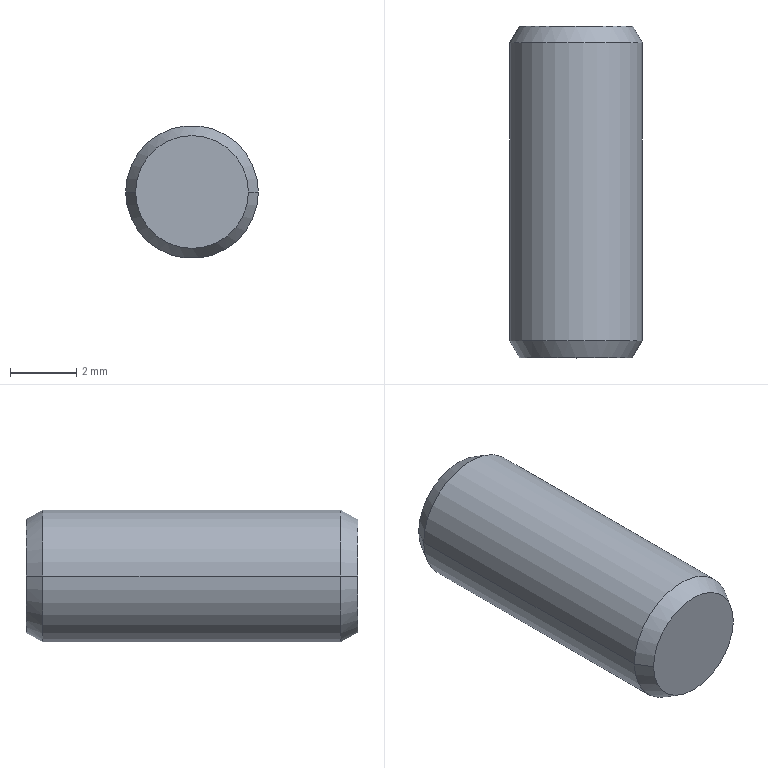Part | STEP file | 1 solid | 8 faces | box 4 x 10 x 4 mm | volume 123.869 mm3 | cone 4 | cylinder 2 | plane 2 | commonest cylinder face diameters 4 x2
STEP:
#1=CARTESIAN_POINT('',(0.,0.,0.));
#2=DIRECTION('',(0.,0.,1.));
#3=DIRECTION('',(1.,0.,0.));
#4=AXIS2_PLACEMENT_3D('',#1,#2,#3);
#5=CARTESIAN_POINT('',(-1.711,0.,0.));
#6=VERTEX_POINT('',#5);
#7=CARTESIAN_POINT('',(1.711,0.,0.));
#8=VERTEX_POINT('',#7);
#9=CARTESIAN_POINT('',(0.,0.,0.));
#10=DIRECTION('',(0.,1.,0.));
#11=DIRECTION('',(-1.,0.,0.));
#12=AXIS2_PLACEMENT_3D('',#9,#10,#11);
#13=CIRCLE('',#12,1.711);
#14=CARTESIAN_POINT('',(0.,0.,0.));
#15=DIRECTION('',(0.,-1.,0.));
#16=DIRECTION('',(1.,0.,0.));
#17=AXIS2_PLACEMENT_3D('',#14,#15,#16);
#18=CONICAL_SURFACE('',#17,1.711,0.5236);
#19=CARTESIAN_POINT('',(3.142,0.));
#20=DIRECTION('',(-1.,0.));
#21=VECTOR('',#20,1.);
#22=LINE('',#19,#21);
#23=(GEOMETRIC_REPRESENTATION_CONTEXT(2)PARAMETRIC_REPRESENTATION_CONTEXT()REPRESENTATION_CONTEXT('',''));
#24=DEFINITIONAL_REPRESENTATION('',(#22),#23);
#25=PCURVE('',#18,#24);
#26=CARTESIAN_POINT('',(0.,0.,0.));
#27=DIRECTION('',(0.,1.,0.));
#28=DIRECTION('',(-1.,0.,0.));
#29=AXIS2_PLACEMENT_3D('',#26,#27,#28);
#30=PLANE('',#29);
#31=CARTESIAN_POINT('',(0.,0.));
#32=DIRECTION('',(1.,0.));
#33=AXIS2_PLACEMENT_2D('',#31,#32);
#34=CIRCLE('',#33,1.711);
#35=(GEOMETRIC_REPRESENTATION_CONTEXT(2)PARAMETRIC_REPRESENTATION_CONTEXT()REPRESENTATION_CONTEXT('',''));
#36=DEFINITIONAL_REPRESENTATION('',(#34),#35);
#37=PCURVE('',#30,#36);
#38=SURFACE_CURVE('',#13,(#25,#37),.PCURVE_S1.);
#39=EDGE_CURVE('',#6,#8,#38,.T.);
#40=ORIENTED_EDGE('',*,*,#39,.F.);
#41=CARTESIAN_POINT('',(-2.,-0.5,0.));
#42=VERTEX_POINT('',#41);
#43=CARTESIAN_POINT('',(-1.711,0.,0.));
#44=DIRECTION('',(-0.5,-0.866,0.));
#45=VECTOR('',#44,1.);
#46=LINE('',#43,#45);
#47=CARTESIAN_POINT('',(3.142,0.));
#48=DIRECTION('',(0.,1.));
#49=VECTOR('',#48,1.);
#50=LINE('',#47,#49);
#51=(GEOMETRIC_REPRESENTATION_CONTEXT(2)PARAMETRIC_REPRESENTATION_CONTEXT()REPRESENTATION_CONTEXT('',''));
#52=DEFINITIONAL_REPRESENTATION('',(#50),#51);
#53=PCURVE('',#18,#52);
#54=CARTESIAN_POINT('',(0.,0.,0.));
#55=DIRECTION('',(0.,-1.,0.));
#56=DIRECTION('',(1.,0.,0.));
#57=AXIS2_PLACEMENT_3D('',#54,#55,#56);
#58=CONICAL_SURFACE('',#57,1.711,0.5236);
#59=CARTESIAN_POINT('',(3.142,0.));
#60=DIRECTION('',(0.,1.));
#61=VECTOR('',#60,1.);
#62=LINE('',#59,#61);
#63=(GEOMETRIC_REPRESENTATION_CONTEXT(2)PARAMETRIC_REPRESENTATION_CONTEXT()REPRESENTATION_CONTEXT('',''));
#64=DEFINITIONAL_REPRESENTATION('',(#62),#63);
#65=PCURVE('',#58,#64);
#66=SURFACE_CURVE('',#46,(#53,#65),.PCURVE_S1.);
#67=EDGE_CURVE('',#6,#42,#66,.T.);
#68=ORIENTED_EDGE('',*,*,#67,.T.);
#69=CARTESIAN_POINT('',(2.,-0.5,0.));
#70=VERTEX_POINT('',#69);
#71=CARTESIAN_POINT('',(0.,-0.5,0.));
#72=DIRECTION('',(0.,-1.,0.));
#73=DIRECTION('',(-1.,0.,0.));
#74=AXIS2_PLACEMENT_3D('',#71,#72,#73);
#75=CIRCLE('',#74,2.);
#76=CARTESIAN_POINT('',(-3.142,0.5));
#77=DIRECTION('',(1.,0.));
#78=VECTOR('',#77,1.);
#79=LINE('',#76,#78);
#80=(GEOMETRIC_REPRESENTATION_CONTEXT(2)PARAMETRIC_REPRESENTATION_CONTEXT()REPRESENTATION_CONTEXT('',''));
#81=DEFINITIONAL_REPRESENTATION('',(#79),#80);
#82=PCURVE('',#18,#81);
#83=CARTESIAN_POINT('',(0.,0.,0.));
#84=DIRECTION('',(0.,1.,0.));
#85=DIRECTION('',(-1.,0.,0.));
#86=AXIS2_PLACEMENT_3D('',#83,#84,#85);
#87=CYLINDRICAL_SURFACE('',#86,2.);
#88=CARTESIAN_POINT('',(6.283,-0.5));
#89=DIRECTION('',(-1.,0.));
#90=VECTOR('',#89,1.);
#91=LINE('',#88,#90);
#92=(GEOMETRIC_REPRESENTATION_CONTEXT(2)PARAMETRIC_REPRESENTATION_CONTEXT()REPRESENTATION_CONTEXT('',''));
#93=DEFINITIONAL_REPRESENTATION('',(#91),#92);
#94=PCURVE('',#87,#93);
#95=SURFACE_CURVE('',#75,(#82,#94),.PCURVE_S1.);
#96=EDGE_CURVE('',#70,#42,#95,.T.);
#97=ORIENTED_EDGE('',*,*,#96,.F.);
#98=CARTESIAN_POINT('',(1.711,0.,0.));
#99=DIRECTION('',(0.5,-0.866,0.));
#100=VECTOR('',#99,1.);
#101=LINE('',#98,#100);
#102=CARTESIAN_POINT('',(0.,0.));
#103=DIRECTION('',(0.,1.));
#104=VECTOR('',#103,1.);
#105=LINE('',#102,#104);
#106=(GEOMETRIC_REPRESENTATION_CONTEXT(2)PARAMETRIC_REPRESENTATION_CONTEXT()REPRESENTATION_CONTEXT('',''));
#107=DEFINITIONAL_REPRESENTATION('',(#105),#106);
#108=PCURVE('',#18,#107);
#109=CARTESIAN_POINT('',(6.283,0.));
#110=DIRECTION('',(0.,1.));
#111=VECTOR('',#110,1.);
#112=LINE('',#109,#111);
#113=(GEOMETRIC_REPRESENTATION_CONTEXT(2)PARAMETRIC_REPRESENTATION_CONTEXT()REPRESENTATION_CONTEXT('',''));
#114=DEFINITIONAL_REPRESENTATION('',(#112),#113);
#115=PCURVE('',#58,#114);
#116=SURFACE_CURVE('',#101,(#108,#115),.PCURVE_S1.);
#117=EDGE_CURVE('',#8,#70,#116,.T.);
#118=ORIENTED_EDGE('',*,*,#117,.F.);
#119=EDGE_LOOP('',(#40,#68,#97,#118));
#120=FACE_BOUND('',#119,.T.);
#121=ADVANCED_FACE('',(#120),#18,.T.);
#122=CARTESIAN_POINT('',(1.7,-10.,0.));
#123=VERTEX_POINT('',#122);
#124=CARTESIAN_POINT('',(-1.7,-10.,0.));
#125=VERTEX_POINT('',#124);
#126=CARTESIAN_POINT('',(0.,-10.,0.));
#127=DIRECTION('',(0.,-1.,0.));
#128=DIRECTION('',(1.,0.,0.));
#129=AXIS2_PLACEMENT_3D('',#126,#127,#128);
#130=CIRCLE('',#129,1.7);
#131=CARTESIAN_POINT('',(0.,-9.48,0.));
#132=DIRECTION('',(0.,1.,0.));
#133=DIRECTION('',(-1.,0.,0.));
#134=AXIS2_PLACEMENT_3D('',#131,#132,#133);
#135=CONICAL_SURFACE('',#134,2.,0.5236);
#136=CARTESIAN_POINT('',(3.142,-0.52));
#137=DIRECTION('',(-1.,0.));
#138=VECTOR('',#137,1.);
#139=LINE('',#136,#138);
#140=(GEOMETRIC_REPRESENTATION_CONTEXT(2)PARAMETRIC_REPRESENTATION_CONTEXT()REPRESENTATION_CONTEXT('',''));
#141=DEFINITIONAL_REPRESENTATION('',(#139),#140);
#142=PCURVE('',#135,#141);
#143=CARTESIAN_POINT('',(0.,-10.,0.));
#144=DIRECTION('',(0.,-1.,0.));
#145=DIRECTION('',(1.,0.,0.));
#146=AXIS2_PLACEMENT_3D('',#143,#144,#145);
#147=PLANE('',#146);
#148=CARTESIAN_POINT('',(0.,0.));
#149=DIRECTION('',(1.,0.));
#150=AXIS2_PLACEMENT_2D('',#148,#149);
#151=CIRCLE('',#150,1.7);
#152=(GEOMETRIC_REPRESENTATION_CONTEXT(2)PARAMETRIC_REPRESENTATION_CONTEXT()REPRESENTATION_CONTEXT('',''));
#153=DEFINITIONAL_REPRESENTATION('',(#151),#152);
#154=PCURVE('',#147,#153);
#155=SURFACE_CURVE('',#130,(#142,#154),.PCURVE_S1.);
#156=EDGE_CURVE('',#123,#125,#155,.T.);
#157=ORIENTED_EDGE('',*,*,#156,.F.);
#158=CARTESIAN_POINT('',(2.,-9.48,0.));
#159=VERTEX_POINT('',#158);
#160=CARTESIAN_POINT('',(2.,-9.48,0.));
#161=DIRECTION('',(0.5,0.866,0.));
#162=VECTOR('',#161,1.);
#163=LINE('',#160,#162);
#164=CARTESIAN_POINT('',(3.142,0.));
#165=DIRECTION('',(0.,1.));
#166=VECTOR('',#165,1.);
#167=LINE('',#164,#166);
#168=(GEOMETRIC_REPRESENTATION_CONTEXT(2)PARAMETRIC_REPRESENTATION_CONTEXT()REPRESENTATION_CONTEXT('',''));
#169=DEFINITIONAL_REPRESENTATION('',(#167),#168);
#170=PCURVE('',#135,#169);
#171=CARTESIAN_POINT('',(0.,-9.48,0.));
#172=DIRECTION('',(0.,1.,0.));
#173=DIRECTION('',(-1.,0.,0.));
#174=AXIS2_PLACEMENT_3D('',#171,#172,#173);
#175=CONICAL_SURFACE('',#174,2.,0.5236);
#176=CARTESIAN_POINT('',(3.142,0.));
#177=DIRECTION('',(0.,1.));
#178=VECTOR('',#177,1.);
#179=LINE('',#176,#178);
#180=(GEOMETRIC_REPRESENTATION_CONTEXT(2)PARAMETRIC_REPRESENTATION_CONTEXT()REPRESENTATION_CONTEXT('',''));
#181=DEFINITIONAL_REPRESENTATION('',(#179),#180);
#182=PCURVE('',#175,#181);
#183=SURFACE_CURVE('',#163,(#170,#182),.PCURVE_S1.);
#184=EDGE_CURVE('',#123,#159,#183,.T.);
#185=ORIENTED_EDGE('',*,*,#184,.T.);
#186=CARTESIAN_POINT('',(-2.,-9.48,0.));
#187=VERTEX_POINT('',#186);
#188=CARTESIAN_POINT('',(0.,-9.48,0.));
#189=DIRECTION('',(0.,1.,0.));
#190=DIRECTION('',(1.,0.,0.));
#191=AXIS2_PLACEMENT_3D('',#188,#189,#190);
#192=CIRCLE('',#191,2.);
#193=CARTESIAN_POINT('',(-3.142,0.));
#194=DIRECTION('',(1.,0.));
#195=VECTOR('',#194,1.);
#196=LINE('',#193,#195);
#197=(GEOMETRIC_REPRESENTATION_CONTEXT(2)PARAMETRIC_REPRESENTATION_CONTEXT()REPRESENTATION_CONTEXT('',''));
#198=DEFINITIONAL_REPRESENTATION('',(#196),#197);
#199=PCURVE('',#135,#198);
#200=CARTESIAN_POINT('',(-3.142,-9.48));
#201=DIRECTION('',(1.,0.));
#202=VECTOR('',#201,1.);
#203=LINE('',#200,#202);
#204=(GEOMETRIC_REPRESENTATION_CONTEXT(2)PARAMETRIC_REPRESENTATION_CONTEXT()REPRESENTATION_CONTEXT('',''));
#205=DEFINITIONAL_REPRESENTATION('',(#203),#204);
#206=PCURVE('',#87,#205);
#207=SURFACE_CURVE('',#192,(#199,#206),.PCURVE_S1.);
#208=EDGE_CURVE('',#187,#159,#207,.T.);
#209=ORIENTED_EDGE('',*,*,#208,.F.);
#210=CARTESIAN_POINT('',(-2.,-9.48,0.));
#211=DIRECTION('',(-0.5,0.866,0.));
#212=VECTOR('',#211,1.);
#213=LINE('',#210,#212);
#214=CARTESIAN_POINT('',(0.,0.));
#215=DIRECTION('',(0.,1.));
#216=VECTOR('',#215,1.);
#217=LINE('',#214,#216);
#218=(GEOMETRIC_REPRESENTATION_CONTEXT(2)PARAMETRIC_REPRESENTATION_CONTEXT()REPRESENTATION_CONTEXT('',''));
#219=DEFINITIONAL_REPRESENTATION('',(#217),#218);
#220=PCURVE('',#135,#219);
#221=CARTESIAN_POINT('',(6.283,0.));
#222=DIRECTION('',(0.,1.));
#223=VECTOR('',#222,1.);
#224=LINE('',#221,#223);
#225=(GEOMETRIC_REPRESENTATION_CONTEXT(2)PARAMETRIC_REPRESENTATION_CONTEXT()REPRESENTATION_CONTEXT('',''));
#226=DEFINITIONAL_REPRESENTATION('',(#224),#225);
#227=PCURVE('',#175,#226);
#228=SURFACE_CURVE('',#213,(#220,#227),.PCURVE_S1.);
#229=EDGE_CURVE('',#125,#187,#228,.T.);
#230=ORIENTED_EDGE('',*,*,#229,.F.);
#231=EDGE_LOOP('',(#157,#185,#209,#230));
#232=FACE_BOUND('',#231,.T.);
#233=ADVANCED_FACE('',(#232),#135,.T.);
#234=ORIENTED_EDGE('',*,*,#208,.T.);
#235=CARTESIAN_POINT('',(2.,0.,0.));
#236=DIRECTION('',(0.,1.,0.));
#237=VECTOR('',#236,1.);
#238=LINE('',#235,#237);
#239=CARTESIAN_POINT('',(3.142,0.));
#240=DIRECTION('',(0.,1.));
#241=VECTOR('',#240,1.);
#242=LINE('',#239,#241);
#243=(GEOMETRIC_REPRESENTATION_CONTEXT(2)PARAMETRIC_REPRESENTATION_CONTEXT()REPRESENTATION_CONTEXT('',''));
#244=DEFINITIONAL_REPRESENTATION('',(#242),#243);
#245=PCURVE('',#87,#244);
#246=CARTESIAN_POINT('',(0.,0.,0.));
#247=DIRECTION('',(0.,1.,0.));
#248=DIRECTION('',(-1.,0.,0.));
#249=AXIS2_PLACEMENT_3D('',#246,#247,#248);
#250=CYLINDRICAL_SURFACE('',#249,2.);
#251=CARTESIAN_POINT('',(3.142,0.));
#252=DIRECTION('',(0.,1.));
#253=VECTOR('',#252,1.);
#254=LINE('',#251,#253);
#255=(GEOMETRIC_REPRESENTATION_CONTEXT(2)PARAMETRIC_REPRESENTATION_CONTEXT()REPRESENTATION_CONTEXT('',''));
#256=DEFINITIONAL_REPRESENTATION('',(#254),#255);
#257=PCURVE('',#250,#256);
#258=SURFACE_CURVE('',#238,(#245,#257),.PCURVE_S1.);
#259=EDGE_CURVE('',#159,#70,#258,.T.);
#260=ORIENTED_EDGE('',*,*,#259,.T.);
#261=ORIENTED_EDGE('',*,*,#96,.T.);
#262=CARTESIAN_POINT('',(-2.,0.,0.));
#263=DIRECTION('',(0.,1.,0.));
#264=VECTOR('',#263,1.);
#265=LINE('',#262,#264);
#266=CARTESIAN_POINT('',(0.,0.));
#267=DIRECTION('',(0.,1.));
#268=VECTOR('',#267,1.);
#269=LINE('',#266,#268);
#270=(GEOMETRIC_REPRESENTATION_CONTEXT(2)PARAMETRIC_REPRESENTATION_CONTEXT()REPRESENTATION_CONTEXT('',''));
#271=DEFINITIONAL_REPRESENTATION('',(#269),#270);
#272=PCURVE('',#87,#271);
#273=CARTESIAN_POINT('',(6.283,0.));
#274=DIRECTION('',(0.,1.));
#275=VECTOR('',#274,1.);
#276=LINE('',#273,#275);
#277=(GEOMETRIC_REPRESENTATION_CONTEXT(2)PARAMETRIC_REPRESENTATION_CONTEXT()REPRESENTATION_CONTEXT('',''));
#278=DEFINITIONAL_REPRESENTATION('',(#276),#277);
#279=PCURVE('',#250,#278);
#280=SURFACE_CURVE('',#265,(#272,#279),.PCURVE_S1.);
#281=EDGE_CURVE('',#187,#42,#280,.T.);
#282=ORIENTED_EDGE('',*,*,#281,.F.);
#283=EDGE_LOOP('',(#234,#260,#261,#282));
#284=FACE_BOUND('',#283,.T.);
#285=ADVANCED_FACE('',(#284),#87,.T.);
#286=CARTESIAN_POINT('',(0.,-10.,0.));
#287=DIRECTION('',(0.,-1.,0.));
#288=DIRECTION('',(1.,0.,0.));
#289=AXIS2_PLACEMENT_3D('',#286,#287,#288);
#290=CIRCLE('',#289,1.7);
#291=CARTESIAN_POINT('',(0.,0.));
#292=DIRECTION('',(1.,0.));
#293=AXIS2_PLACEMENT_2D('',#291,#292);
#294=CIRCLE('',#293,1.7);
#295=(GEOMETRIC_REPRESENTATION_CONTEXT(2)PARAMETRIC_REPRESENTATION_CONTEXT()REPRESENTATION_CONTEXT('',''));
#296=DEFINITIONAL_REPRESENTATION('',(#294),#295);
#297=PCURVE('',#147,#296);
#298=CARTESIAN_POINT('',(9.425,-0.52));
#299=DIRECTION('',(-1.,0.));
#300=VECTOR('',#299,1.);
#301=LINE('',#298,#300);
#302=(GEOMETRIC_REPRESENTATION_CONTEXT(2)PARAMETRIC_REPRESENTATION_CONTEXT()REPRESENTATION_CONTEXT('',''));
#303=DEFINITIONAL_REPRESENTATION('',(#301),#302);
#304=PCURVE('',#175,#303);
#305=SURFACE_CURVE('',#290,(#297,#304),.PCURVE_S1.);
#306=EDGE_CURVE('',#125,#123,#305,.T.);
#307=ORIENTED_EDGE('',*,*,#306,.T.);
#308=ORIENTED_EDGE('',*,*,#156,.T.);
#309=EDGE_LOOP('',(#307,#308));
#310=FACE_BOUND('',#309,.T.);
#311=ADVANCED_FACE('',(#310),#147,.T.);
#312=ORIENTED_EDGE('',*,*,#259,.F.);
#313=CARTESIAN_POINT('',(0.,-9.48,0.));
#314=DIRECTION('',(0.,1.,0.));
#315=DIRECTION('',(1.,0.,0.));
#316=AXIS2_PLACEMENT_3D('',#313,#314,#315);
#317=CIRCLE('',#316,2.);
#318=CARTESIAN_POINT('',(3.142,-9.48));
#319=DIRECTION('',(1.,0.));
#320=VECTOR('',#319,1.);
#321=LINE('',#318,#320);
#322=(GEOMETRIC_REPRESENTATION_CONTEXT(2)PARAMETRIC_REPRESENTATION_CONTEXT()REPRESENTATION_CONTEXT('',''));
#323=DEFINITIONAL_REPRESENTATION('',(#321),#322);
#324=PCURVE('',#250,#323);
#325=CARTESIAN_POINT('',(3.142,0.));
#326=DIRECTION('',(1.,0.));
#327=VECTOR('',#326,1.);
#328=LINE('',#325,#327);
#329=(GEOMETRIC_REPRESENTATION_CONTEXT(2)PARAMETRIC_REPRESENTATION_CONTEXT()REPRESENTATION_CONTEXT('',''));
#330=DEFINITIONAL_REPRESENTATION('',(#328),#329);
#331=PCURVE('',#175,#330);
#332=SURFACE_CURVE('',#317,(#324,#331),.PCURVE_S1.);
#333=EDGE_CURVE('',#159,#187,#332,.T.);
#334=ORIENTED_EDGE('',*,*,#333,.T.);
#335=ORIENTED_EDGE('',*,*,#281,.T.);
#336=CARTESIAN_POINT('',(0.,-0.5,0.));
#337=DIRECTION('',(0.,-1.,0.));
#338=DIRECTION('',(-1.,0.,0.));
#339=AXIS2_PLACEMENT_3D('',#336,#337,#338);
#340=CIRCLE('',#339,2.);
#341=CARTESIAN_POINT('',(6.283,-0.5));
#342=DIRECTION('',(-1.,0.));
#343=VECTOR('',#342,1.);
#344=LINE('',#341,#343);
#345=(GEOMETRIC_REPRESENTATION_CONTEXT(2)PARAMETRIC_REPRESENTATION_CONTEXT()REPRESENTATION_CONTEXT('',''));
#346=DEFINITIONAL_REPRESENTATION('',(#344),#345);
#347=PCURVE('',#250,#346);
#348=CARTESIAN_POINT('',(3.142,0.5));
#349=DIRECTION('',(1.,0.));
#350=VECTOR('',#349,1.);
#351=LINE('',#348,#350);
#352=(GEOMETRIC_REPRESENTATION_CONTEXT(2)PARAMETRIC_REPRESENTATION_CONTEXT()REPRESENTATION_CONTEXT('',''));
#353=DEFINITIONAL_REPRESENTATION('',(#351),#352);
#354=PCURVE('',#58,#353);
#355=SURFACE_CURVE('',#340,(#347,#354),.PCURVE_S1.);
#356=EDGE_CURVE('',#42,#70,#355,.T.);
#357=ORIENTED_EDGE('',*,*,#356,.T.);
#358=EDGE_LOOP('',(#312,#334,#335,#357));
#359=FACE_BOUND('',#358,.T.);
#360=ADVANCED_FACE('',(#359),#250,.T.);
#361=CARTESIAN_POINT('',(0.,0.,0.));
#362=DIRECTION('',(0.,1.,0.));
#363=DIRECTION('',(-1.,0.,0.));
#364=AXIS2_PLACEMENT_3D('',#361,#362,#363);
#365=CIRCLE('',#364,1.711);
#366=CARTESIAN_POINT('',(0.,0.));
#367=DIRECTION('',(1.,0.));
#368=AXIS2_PLACEMENT_2D('',#366,#367);
#369=CIRCLE('',#368,1.711);
#370=(GEOMETRIC_REPRESENTATION_CONTEXT(2)PARAMETRIC_REPRESENTATION_CONTEXT()REPRESENTATION_CONTEXT('',''));
#371=DEFINITIONAL_REPRESENTATION('',(#369),#370);
#372=PCURVE('',#30,#371);
#373=CARTESIAN_POINT('',(9.425,0.));
#374=DIRECTION('',(-1.,0.));
#375=VECTOR('',#374,1.);
#376=LINE('',#373,#375);
#377=(GEOMETRIC_REPRESENTATION_CONTEXT(2)PARAMETRIC_REPRESENTATION_CONTEXT()REPRESENTATION_CONTEXT('',''));
#378=DEFINITIONAL_REPRESENTATION('',(#376),#377);
#379=PCURVE('',#58,#378);
#380=SURFACE_CURVE('',#365,(#372,#379),.PCURVE_S1.);
#381=EDGE_CURVE('',#8,#6,#380,.T.);
#382=ORIENTED_EDGE('',*,*,#381,.T.);
#383=ORIENTED_EDGE('',*,*,#39,.T.);
#384=EDGE_LOOP('',(#382,#383));
#385=FACE_BOUND('',#384,.T.);
#386=ADVANCED_FACE('',(#385),#30,.T.);
#387=ORIENTED_EDGE('',*,*,#184,.F.);
#388=ORIENTED_EDGE('',*,*,#306,.F.);
#389=ORIENTED_EDGE('',*,*,#229,.T.);
#390=ORIENTED_EDGE('',*,*,#333,.F.);
#391=EDGE_LOOP('',(#387,#388,#389,#390));
#392=FACE_BOUND('',#391,.T.);
#393=ADVANCED_FACE('',(#392),#175,.T.);
#394=ORIENTED_EDGE('',*,*,#67,.F.);
#395=ORIENTED_EDGE('',*,*,#381,.F.);
#396=ORIENTED_EDGE('',*,*,#117,.T.);
#397=ORIENTED_EDGE('',*,*,#356,.F.);
#398=EDGE_LOOP('',(#394,#395,#396,#397));
#399=FACE_BOUND('',#398,.T.);
#400=ADVANCED_FACE('',(#399),#58,.T.);
#401=CLOSED_SHELL('',(#121,#233,#285,#311,#360,#386,#393,#400));
#402=MANIFOLD_SOLID_BREP('',#401);
#403=(LENGTH_UNIT()NAMED_UNIT(*)SI_UNIT(.MILLI.,.METRE.));
#404=UNCERTAINTY_MEASURE_WITH_UNIT(LENGTH_MEASURE(0.0000001),#403,'','');
#405=(NAMED_UNIT(*)PLANE_ANGLE_UNIT()SI_UNIT($,.RADIAN.));
#406=(NAMED_UNIT(*)SI_UNIT($,.STERADIAN.)SOLID_ANGLE_UNIT());
#407=(GEOMETRIC_REPRESENTATION_CONTEXT(3)GLOBAL_UNCERTAINTY_ASSIGNED_CONTEXT((#404))GLOBAL_UNIT_ASSIGNED_CONTEXT((#403,#405,#406))REPRESENTATION_CONTEXT('',''));
#408=ADVANCED_BREP_SHAPE_REPRESENTATION('',(#4,#402),#407);